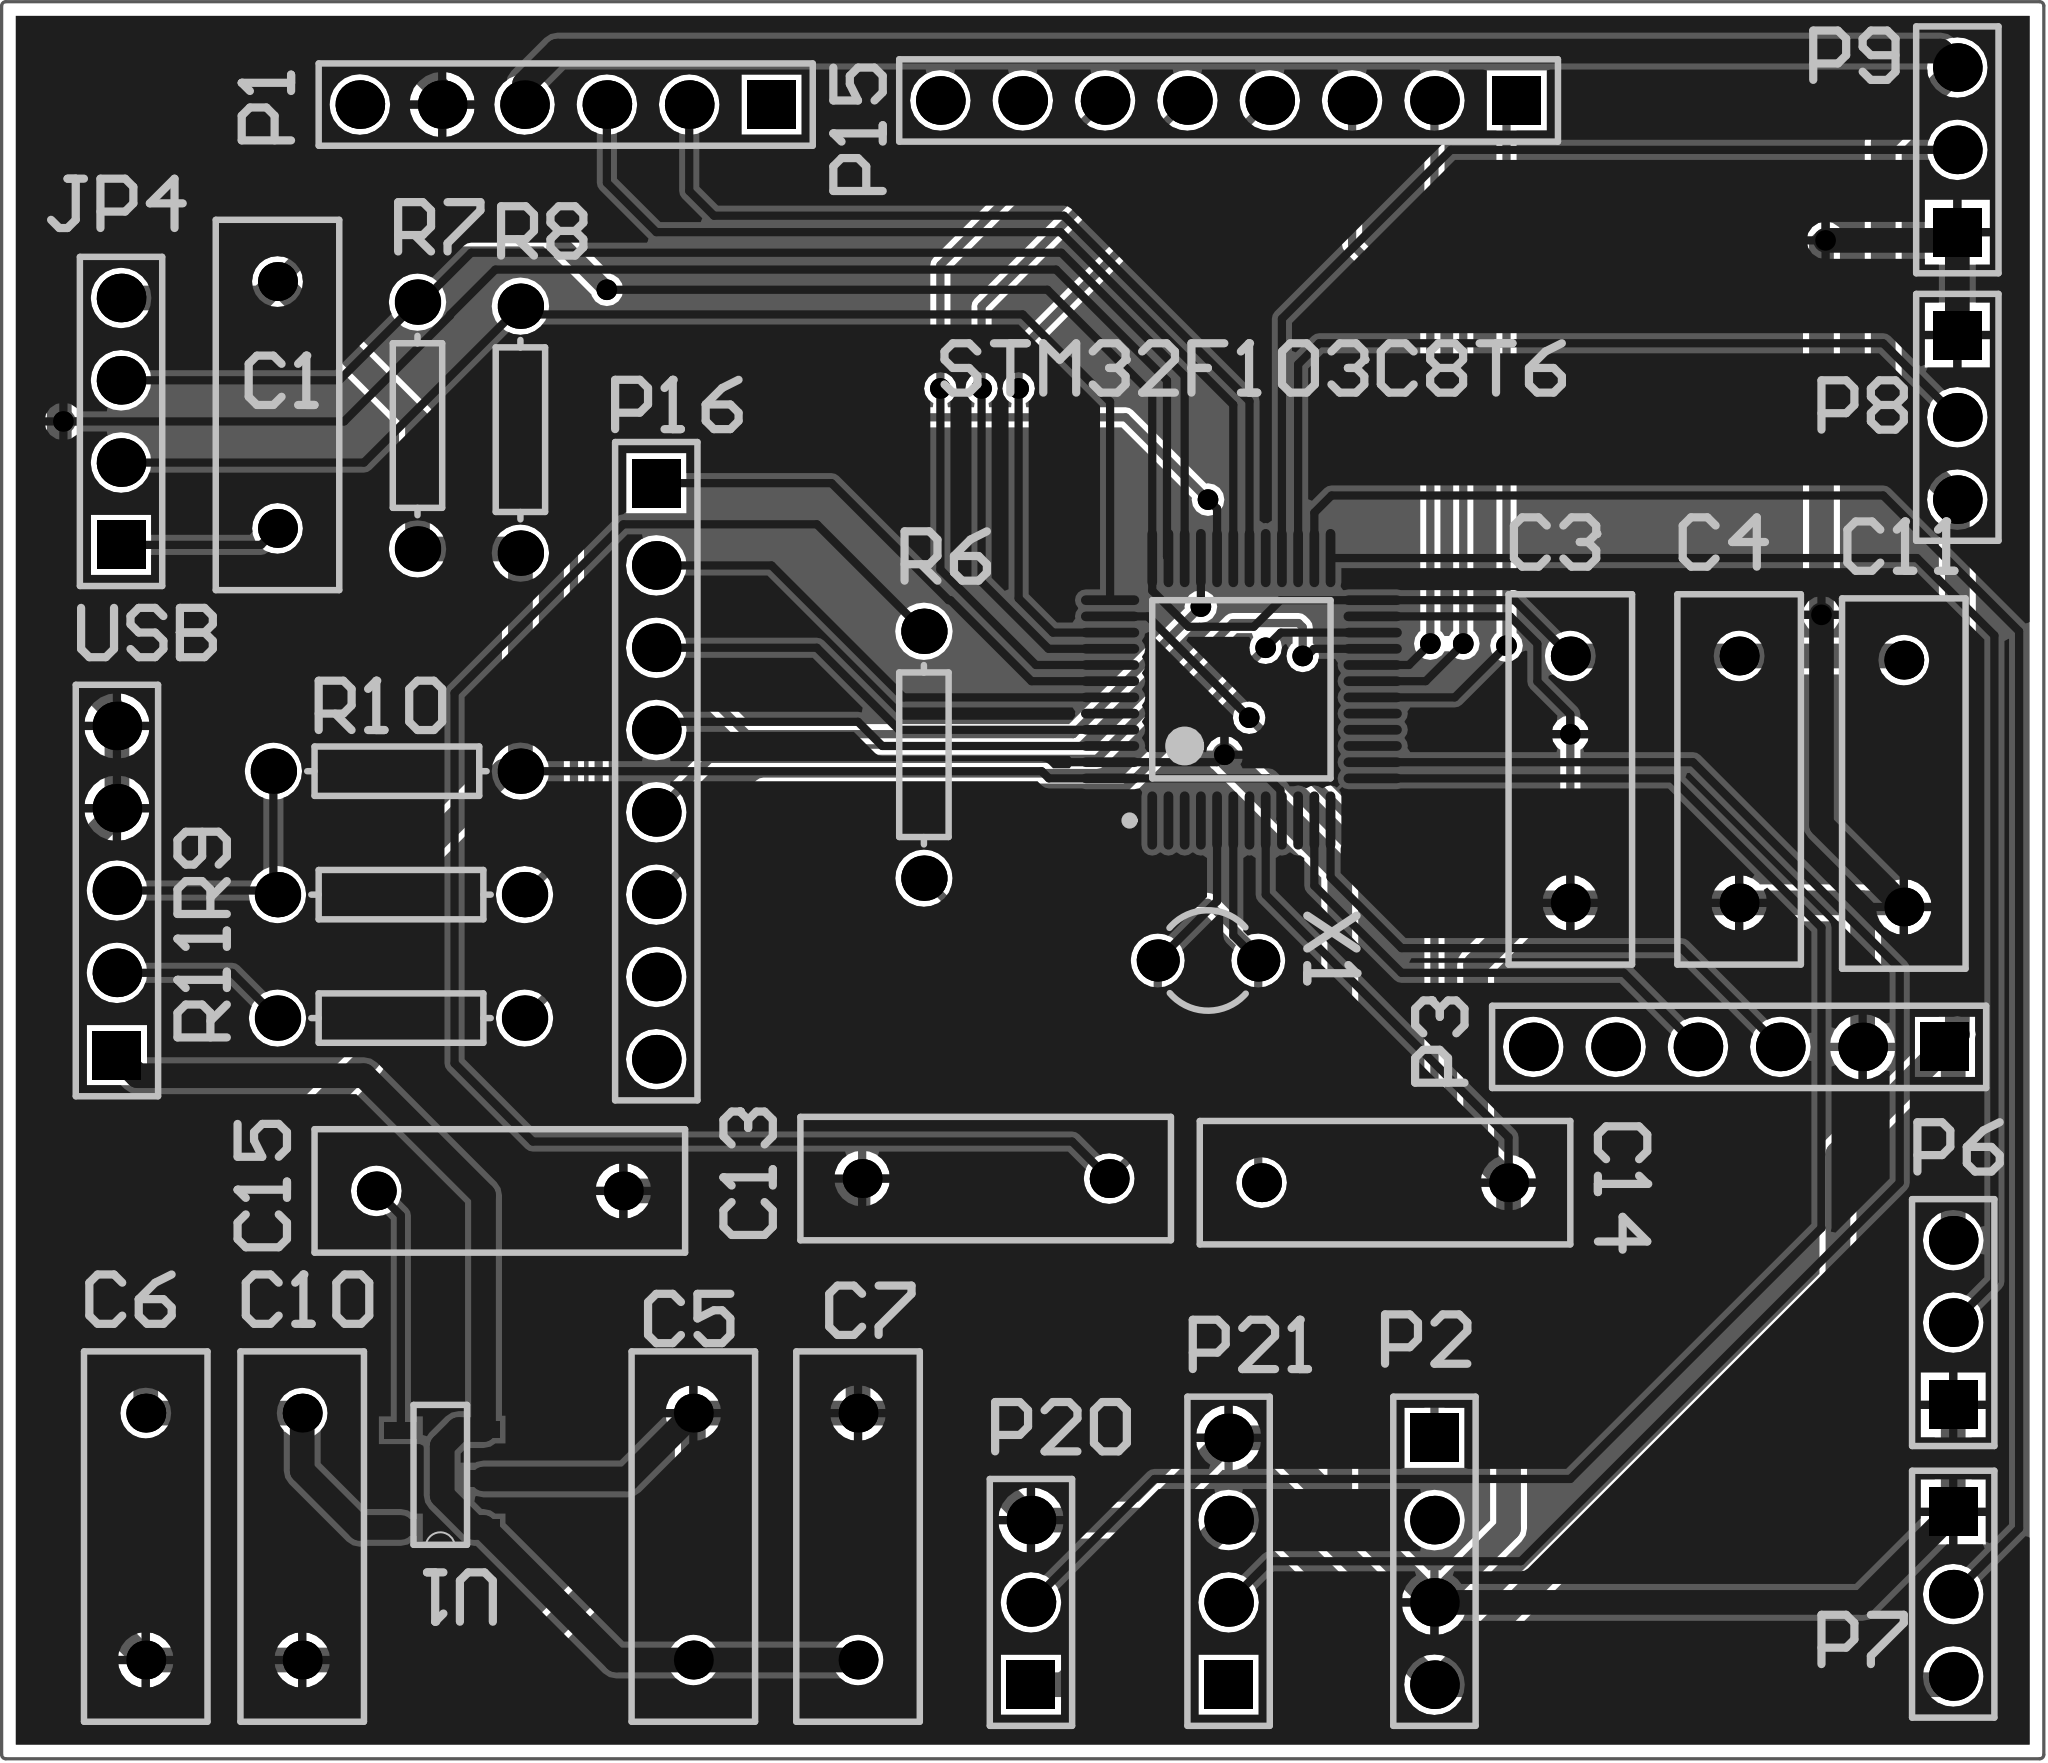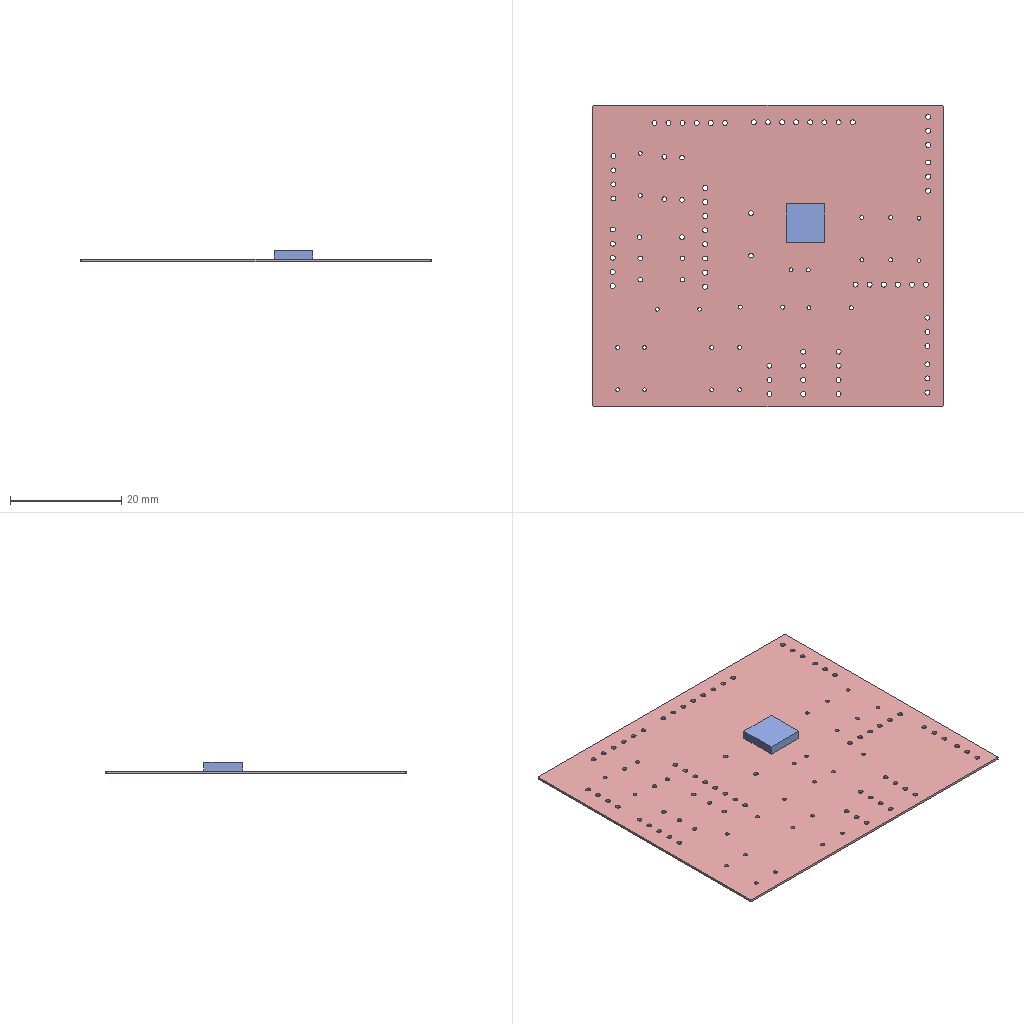Circuit board layout | Altium Designer | box 63 x 54.2 x 2 mm
Layer stack:
# Altium Designer layer stack of  (unit mm; dielectric type: 0 none, 1 core, 2 prepreg, 3 surface material)
index,name,kind,layer,copper_thickness_mm,dielectric_type,dielectric_thickness_mm,dielectric_material,dielectric_constant
0,Top Paste,other,,,,,,
1,Top Overlay,other,,,,,,
2,Top Solder,dielectric,,,3,0.0102,Solder Resist,3.5
3,Top Layer,copper,Top Layer,0.0356,,,,
4,Dielectric 1,dielectric,,,0,0.32,FR-4,4.8
5,Bottom Layer,copper,Bottom Layer,0.0356,,,,
6,Bottom Solder,dielectric,,,3,0.0102,Solder Resist,3.5
7,Bottom Overlay,other,,,,,,
8,Bottom Paste,other,,,,,,
# drill layer pairs: low layer,high layer
drill_pair,Top Layer,Bottom Layer
Part placement:
Designator,Comment,Layer,Footprint,Center-X(mm),Center-Y(mm),Rotation
U1,EM6211,TopLayer,ME6211C28M5G,53.213,47.131,180
X1,XTAL,TopLayer,R38,76.835,63.119,270
USB,USB-5P,TopLayer,HDR1X5,43.18,65.278,90
STM32F103C8T6,STM32F103C8T6,TopLayer,PCBComponent_1,77.865,71.489,90
R11,Res1,TopLayer,AXIAL-0.3,51.943,61.341,180
R10,Res1,TopLayer,AXIAL-0.3,51.816,68.961,360
R9,Res1,TopLayer,AXIAL-0.3,51.943,65.151,180
R8,Res1,TopLayer,AXIAL-0.3,55.626,79.502,90
R7,Res1,TopLayer,AXIAL-0.3,52.451,79.629,90
R6,Res1,TopLayer,AXIAL-0.3,68.072,69.469,90
P21,OLED,TopLayer,HDR1X4,77.47,44.577,90
P20,DHT11,TopLayer,HDR1X3,71.374,43.307,90
P16,Header 8,TopLayer,HDR1X8,59.817,68.961,270
P15,Header 8,TopLayer,HDR1X8,77.47,89.662,180
P9,TTP233,TopLayer,HDR1X3,99.949,88.138,90
P8,TTP233,TopLayer,HDR1X3,99.949,79.883,270
P7,TTP233,TopLayer,HDR1X3,99.822,43.561,270
P6,TTP233,TopLayer,HDR1X3,99.822,51.943,90
P3,VL53L0X,TopLayer,HDR1X6,93.218,60.452,180
P2,Header 4,TopLayer,HDR1X4,83.82,44.577,270
P1,Header 6,TopLayer,HDR1X6,57.023,89.535,180
JP4,Header 4,TopLayer,HDR1X4,43.307,79.756,90
C15,223,TopLayer,RAD-0.3,54.991,56.007,180
C14,Cap,TopLayer,RAD-0.3,82.296,56.261,360
C13,Cap,TopLayer,RAD-0.3,69.977,56.388,180
C11,Cap,TopLayer,RAD-0.3,98.298,68.58,90
C10,104,TopLayer,RAD-0.3,48.895,45.339,90
C7,104,TopLayer,RAD-0.3,66.04,45.339,270
C6,105,TopLayer,RAD-0.3,44.069,45.339,90
C5,105,TopLayer,RAD-0.3,60.96,45.339,270
C4,Cap,TopLayer,RAD-0.3,93.218,68.707,90
C3,Cap,TopLayer,RAD-0.3,88.011,68.707,90
C1,104,TopLayer,RAD-0.3,48.133,80.264,90
Pad and via stacks:
# Altium Designer via and pad stacks of  (unit mm). Each distinct definition once, with the count of objects using it.
# via: kind,start_layer,end_layer,hole_mm,diameter_mm,mode(0 simple;1 top-mid-bottom;2 full stack),diameter_per_layer,count,example_net
# pad: kind,layer,hole_mm,hole_type(0 round;1 square;2 slot),plating,top_size,top_shape(1 round;2 rect;3 octagon;9 rounded rect),mid_size,bottom_size,mode,footprint,size_per_layer,count,example
pad,Multi-Layer,0.9,0,plated,1.5x1.5,2,1.5x1.5,1.5x1.5,0,HDR1X6,,2,P1.1
pad,Multi-Layer,0.9,0,plated,1.5x1.5,1,1.5x1.5,1.5x1.5,0,HDR1X6,,10,P1.2
pad,Multi-Layer,0.9,0,plated,1.5x1.5,1,1.5x1.5,1.5x1.5,0,HDR1X4,,9,P2.4
pad,Multi-Layer,0.9,0,plated,1.5x1.5,2,1.5x1.5,1.5x1.5,0,HDR1X4,,3,P2.1
pad,Multi-Layer,0.9,0,plated,1.5x1.5,2,1.5x1.5,1.5x1.5,0,HDR1X3,,5,P20.1
pad,Multi-Layer,0.9,0,plated,1.5x1.5,1,1.5x1.5,1.5x1.5,0,HDR1X3,,10,P20.2
pad,Multi-Layer,0.9,0,plated,1.5x1.5,2,1.5x1.5,1.5x1.5,0,HDR1X8,,2,P15.1
pad,Multi-Layer,0.9,0,plated,1.5x1.5,1,1.5x1.5,1.5x1.5,0,HDR1X8,,14,P15.2
pad,Multi-Layer,0.7,0,plated,1.2x1.2,1,1.2x1.2,1.2x1.2,0,RAD-0.3,,22,C13.2
pad,Multi-Layer,0.85,0,plated,1.4x1.4,1,1.4x1.4,1.4x1.4,0,AXIAL-0.3,,12,R6.2
pad,Multi-Layer,0.7,0,plated,1.3x1.3,1,1.3x1.3,1.3x1.3,0,R38,,2,X1.1
pad,Multi-Layer,0.9,0,plated,1.5x1.5,1,1.5x1.5,1.5x1.5,0,HDR1X5,,4,USB.5
pad,Multi-Layer,0.9,0,plated,1.5x1.5,2,1.5x1.5,1.5x1.5,0,HDR1X5,,1,USB.1
pad,Top Layer,0,0,plated,1x0.5,2,1x0.5,1x0.5,0,ME6211C28M5G,,5,U1.5
pad,Top Layer,0,0,plated,0.3x1.8,1,0.3x1.8,0.3x1.8,0,PCBComponent_1,,48,STM32F103C8T6.36
via,Top Layer,Bottom Layer,0.381,0.635,0,,17,GND
Copper pours:
name,layer,net,type(0 solid;1 hatched;2 none)
Top Layer-No Net,Top Layer,GND,0
Top Layer-No Net,Bottom Layer,GND,0
Design rules, without the lines most boards share:
# Altium Designer design rules of  (exported by Altium Designer, unit mm)
# columns: name | kind | enabled | priority | scope1 | scope2 | descriptor | typed fields (field=value)
Clearance | 0 | enabled | 1 | All | All | Clearance Constraint (Gap=7mil) (All),(All) | gap=0.1778
PlaneConnect | 6 | enabled | 1 | All | All | Power Plane Connect Rule(Relief Connect )(Expansion=20mil) (Conductor Width=10mil) (Air Gap=10mil) (Entries=4) (All) | relief_conductor_width=0.254 relief_entries=4 relief_expansion=0.508
PolygonConnect | 20 | enabled | 1 | All | All | Polygon Connect Rule(Relief Connect )(Conductor Width=10mil) (Relief Angle=90 Angle) (Entries=4) (Air Gap Width=10mil) (All),(All) | connect_style(0=relief,1=direct,2=none)=0 relief_conductor_width=0.254 relief_entries=4
Width | 2 | enabled | 1 | All | All | Width Constraint (Min=10mil) (Max=50mil) (Preferred=20mil) (All) |
RoutingVias | 11 | enabled | 1 | All | All | Routing Via (MinHoleWidth=28mil) (MaxHoleWidth=28mil) (PreferredHoleWidth=28mil) (MinWidth=50mil) (MaxWidth=50mil) (PreferedWidth=50mil) (All) | via_min_hole=0.7112 via_max_hole=0.7112 via_preferred_diameter=1.27 via_preferred_hole=0.7112
PasteMaskExpansion | 14 | enabled | 1 | All | All | Paste Mask Expansion (Expansion =0mil) (All) | expansion=0
SolderMaskExpansion | 13 | enabled | 1 | All | All | Solder Mask Expansion (Expansion =4mil) (All) | expansion=0.1016
DiffPairsRouting | 51 | enabled | 1 | All | All | Differential Pairs Uncoupled Length using the Gap Constraints (Min=10mil) (Max=10mil) (Prefered=10mil)  and Width Constraints (Min=15mil) (Max=15mil) (Prefered=15mil) (All) |
HoleToHoleClearance | 52 | enabled | 1 | All | All | Hole To Hole Clearance (Gap=10mil) (All),(All) | gap=0.254
Classes set for this board:
# Altium Designer classes of  (member kind: 0 net, 1 component, 2 from-to, 3 pad, 4 layer, 5 differential pair, 6 design channel, 7 polygon, 8 structure, 9 xSignal)
# columns: class name | member kind | superclass | members
Sheet1 | 1 | no | C1; C3; C4; C5; C6; C7; C10; C11; C13; C14; C15; JP4; P1; P2; P3; P6; P7; P8; P9; P15; P16; P20; P21; R6; R7; R8; R9; R10; R11; STM32F103C8T6; USB; X1; U1;